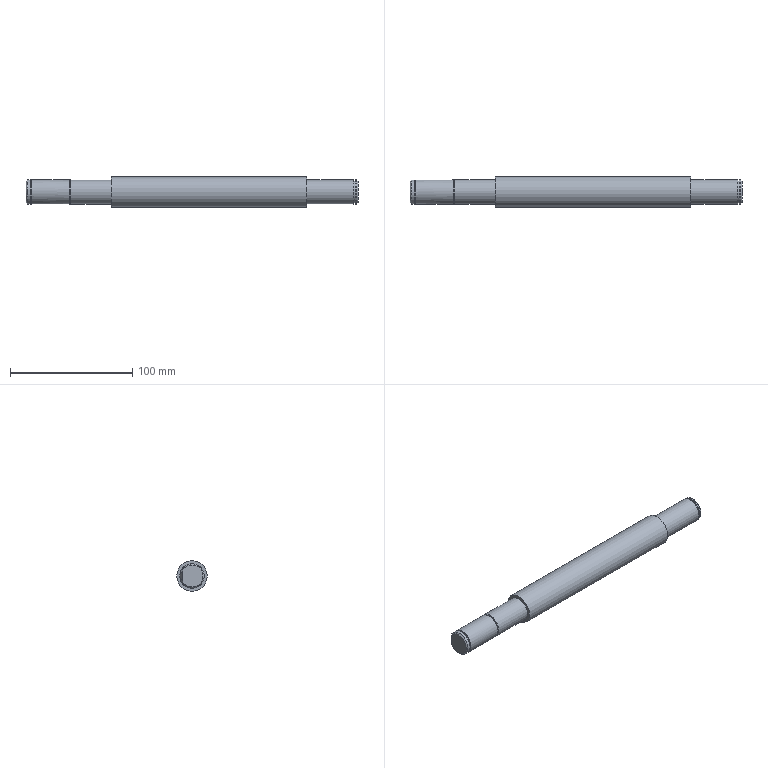Part | STEP file | Shaft1 | 1 solid | 25 faces | box 272 x 25 x 25 mm | volume 113038 mm3 | plane 13 | cylinder 10 | cone 2 | commonest cylinder face diameters 20 x6 18.35 x3 25 x1